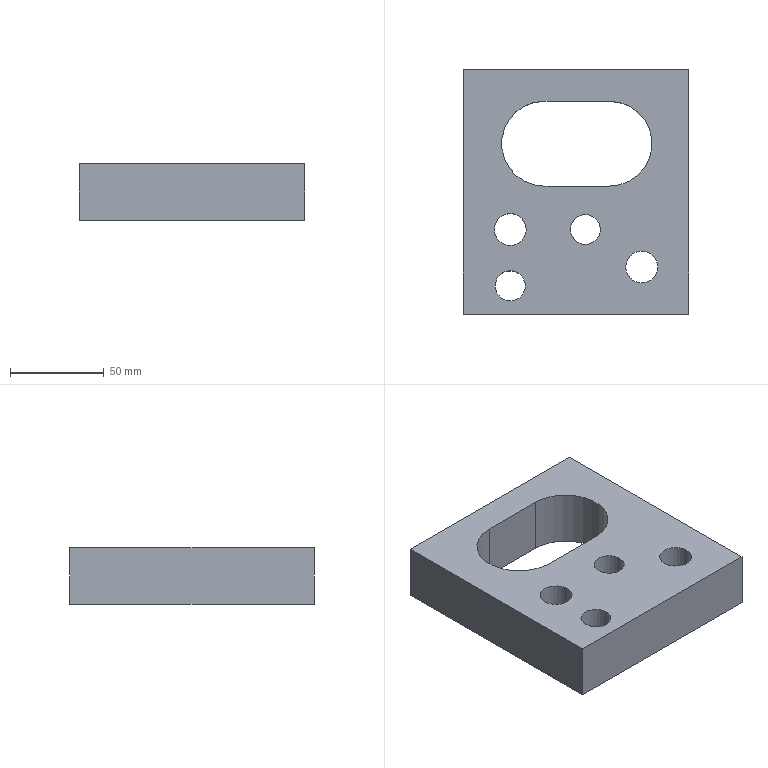Part | NX | features solid 2 | 1 solid | 18 faces | box 120 x 130 x 30 mm | volume 337905 mm3 | plane 10 | cylinder 8 | commonest cylinder face diameters 16 x2 17 x2 26 x2 45.1 x2
STEP:
#1=CARTESIAN_POINT('',(-328.,695.,180.));
#2=VERTEX_POINT('',#1);
#3=CARTESIAN_POINT('',(-320.,695.,180.));
#4=DIRECTION('',(0.,0.,-1.));
#5=DIRECTION('',(-1.,0.,0.));
#6=AXIS2_PLACEMENT_3D('',#3,#4,#5);
#7=CIRCLE('',#6,8.);
#8=EDGE_CURVE('',#2,#2,#7,.T.);
#9=ORIENTED_EDGE('',*,*,#8,.T.);
#10=EDGE_LOOP('',(#9));
#11=FACE_BOUND('',#10,.T.);
#12=CARTESIAN_POINT('',(-225.,680.,180.));
#13=VERTEX_POINT('',#12);
#14=CARTESIAN_POINT('',(-225.,810.,180.));
#15=VERTEX_POINT('',#14);
#16=CARTESIAN_POINT('',(-225.,680.,180.));
#17=DIRECTION('',(0.,1.,0.));
#18=VECTOR('',#17,1000.);
#19=LINE('',#16,#18);
#20=EDGE_CURVE('',#13,#15,#19,.T.);
#21=ORIENTED_EDGE('',*,*,#20,.T.);
#22=CARTESIAN_POINT('',(-345.,810.,180.));
#23=VERTEX_POINT('',#22);
#24=CARTESIAN_POINT('',(-385.,810.,180.));
#25=DIRECTION('',(1.,0.,0.));
#26=VECTOR('',#25,1000.);
#27=LINE('',#24,#26);
#28=EDGE_CURVE('',#23,#15,#27,.T.);
#29=ORIENTED_EDGE('',*,*,#28,.F.);
#30=CARTESIAN_POINT('',(-345.,680.,180.));
#31=VERTEX_POINT('',#30);
#32=CARTESIAN_POINT('',(-345.,810.,180.));
#33=DIRECTION('',(0.,1.,0.));
#34=VECTOR('',#33,1000.);
#35=LINE('',#32,#34);
#36=EDGE_CURVE('',#31,#23,#35,.T.);
#37=ORIENTED_EDGE('',*,*,#36,.F.);
#38=CARTESIAN_POINT('',(-385.,680.,180.));
#39=DIRECTION('',(1.,0.,0.));
#40=VECTOR('',#39,1000.);
#41=LINE('',#38,#40);
#42=EDGE_CURVE('',#31,#13,#41,.T.);
#43=ORIENTED_EDGE('',*,*,#42,.T.);
#44=EDGE_LOOP('',(#21,#29,#37,#43));
#45=FACE_BOUND('',#44,.T.);
#46=CARTESIAN_POINT('',(-311.5,725.,180.));
#47=VERTEX_POINT('',#46);
#48=CARTESIAN_POINT('',(-320.,725.,180.));
#49=DIRECTION('',(0.,0.,1.));
#50=DIRECTION('',(1.,0.,0.));
#51=AXIS2_PLACEMENT_3D('',#48,#49,#50);
#52=CIRCLE('',#51,8.5);
#53=EDGE_CURVE('',#47,#47,#52,.T.);
#54=ORIENTED_EDGE('',*,*,#53,.F.);
#55=EDGE_LOOP('',(#54));
#56=FACE_BOUND('',#55,.T.);
#57=CARTESIAN_POINT('',(-241.5,705.,180.));
#58=VERTEX_POINT('',#57);
#59=CARTESIAN_POINT('',(-250.,705.,180.));
#60=DIRECTION('',(0.,0.,1.));
#61=DIRECTION('',(1.,0.,0.));
#62=AXIS2_PLACEMENT_3D('',#59,#60,#61);
#63=CIRCLE('',#62,8.5);
#64=EDGE_CURVE('',#58,#58,#63,.T.);
#65=ORIENTED_EDGE('',*,*,#64,.F.);
#66=EDGE_LOOP('',(#65));
#67=FACE_BOUND('',#66,.T.);
#68=CARTESIAN_POINT('',(-288.,725.,180.));
#69=VERTEX_POINT('',#68);
#70=CARTESIAN_POINT('',(-280.,725.,180.));
#71=DIRECTION('',(0.,0.,-1.));
#72=DIRECTION('',(-1.,0.,0.));
#73=AXIS2_PLACEMENT_3D('',#70,#71,#72);
#74=CIRCLE('',#73,8.);
#75=EDGE_CURVE('',#69,#69,#74,.T.);
#76=ORIENTED_EDGE('',*,*,#75,.T.);
#77=EDGE_LOOP('',(#76));
#78=FACE_BOUND('',#77,.T.);
#79=CARTESIAN_POINT('',(-267.044,748.16,180.));
#80=VERTEX_POINT('',#79);
#81=CARTESIAN_POINT('',(-267.044,793.26,180.));
#82=VERTEX_POINT('',#81);
#83=CARTESIAN_POINT('',(-267.044,770.71,180.));
#84=DIRECTION('',(0.,0.,1.));
#85=DIRECTION('',(0.,-1.,0.));
#86=AXIS2_PLACEMENT_3D('',#83,#84,#85);
#87=CIRCLE('',#86,22.55);
#88=EDGE_CURVE('',#80,#82,#87,.T.);
#89=ORIENTED_EDGE('',*,*,#88,.F.);
#90=CARTESIAN_POINT('',(-302.055,748.16,180.));
#91=VERTEX_POINT('',#90);
#92=CARTESIAN_POINT('',(-267.044,748.16,180.));
#93=DIRECTION('',(-1.,0.,0.));
#94=VECTOR('',#93,1000.);
#95=LINE('',#92,#94);
#96=EDGE_CURVE('',#80,#91,#95,.T.);
#97=ORIENTED_EDGE('',*,*,#96,.T.);
#98=CARTESIAN_POINT('',(-302.055,793.26,180.));
#99=VERTEX_POINT('',#98);
#100=CARTESIAN_POINT('',(-302.055,770.71,180.));
#101=DIRECTION('',(0.,0.,1.));
#102=DIRECTION('',(0.,-1.,0.));
#103=AXIS2_PLACEMENT_3D('',#100,#101,#102);
#104=CIRCLE('',#103,22.55);
#105=EDGE_CURVE('',#99,#91,#104,.T.);
#106=ORIENTED_EDGE('',*,*,#105,.F.);
#107=CARTESIAN_POINT('',(-302.055,793.26,180.));
#108=DIRECTION('',(1.,0.,0.));
#109=VECTOR('',#108,1000.);
#110=LINE('',#107,#109);
#111=EDGE_CURVE('',#99,#82,#110,.T.);
#112=ORIENTED_EDGE('',*,*,#111,.T.);
#113=EDGE_LOOP('',(#89,#97,#106,#112));
#114=FACE_BOUND('',#113,.T.);
#115=CARTESIAN_POINT('',(-225.,810.,180.));
#116=DIRECTION('',(0.,0.,-1.));
#117=DIRECTION('',(0.,1.,0.));
#118=AXIS2_PLACEMENT_3D('',#115,#116,#117);
#119=PLANE('',#118);
#120=ADVANCED_FACE('',(#11,#45,#56,#67,#78,#114),#119,.F.);
#121=CARTESIAN_POINT('',(-312.,695.,150.));
#122=VERTEX_POINT('',#121);
#123=CARTESIAN_POINT('',(-320.,695.,150.));
#124=DIRECTION('',(0.,0.,1.));
#125=DIRECTION('',(1.,0.,0.));
#126=AXIS2_PLACEMENT_3D('',#123,#124,#125);
#127=CIRCLE('',#126,8.);
#128=EDGE_CURVE('',#122,#122,#127,.T.);
#129=ORIENTED_EDGE('',*,*,#128,.T.);
#130=EDGE_LOOP('',(#129));
#131=FACE_BOUND('',#130,.T.);
#132=CARTESIAN_POINT('',(-225.,680.,150.));
#133=VERTEX_POINT('',#132);
#134=CARTESIAN_POINT('',(-225.,810.,150.));
#135=VERTEX_POINT('',#134);
#136=CARTESIAN_POINT('',(-225.,680.,150.));
#137=DIRECTION('',(0.,1.,0.));
#138=VECTOR('',#137,1000.);
#139=LINE('',#136,#138);
#140=EDGE_CURVE('',#133,#135,#139,.T.);
#141=ORIENTED_EDGE('',*,*,#140,.F.);
#142=CARTESIAN_POINT('',(-345.,680.,150.));
#143=VERTEX_POINT('',#142);
#144=CARTESIAN_POINT('',(-385.,680.,150.));
#145=DIRECTION('',(1.,0.,0.));
#146=VECTOR('',#145,1000.);
#147=LINE('',#144,#146);
#148=EDGE_CURVE('',#143,#133,#147,.T.);
#149=ORIENTED_EDGE('',*,*,#148,.F.);
#150=CARTESIAN_POINT('',(-345.,810.,150.));
#151=VERTEX_POINT('',#150);
#152=CARTESIAN_POINT('',(-345.,810.,150.));
#153=DIRECTION('',(0.,1.,0.));
#154=VECTOR('',#153,1000.);
#155=LINE('',#152,#154);
#156=EDGE_CURVE('',#143,#151,#155,.T.);
#157=ORIENTED_EDGE('',*,*,#156,.T.);
#158=CARTESIAN_POINT('',(-385.,810.,150.));
#159=DIRECTION('',(1.,0.,0.));
#160=VECTOR('',#159,1000.);
#161=LINE('',#158,#160);
#162=EDGE_CURVE('',#151,#135,#161,.T.);
#163=ORIENTED_EDGE('',*,*,#162,.T.);
#164=EDGE_LOOP('',(#141,#149,#157,#163));
#165=FACE_BOUND('',#164,.T.);
#166=CARTESIAN_POINT('',(-307.,725.,150.));
#167=VERTEX_POINT('',#166);
#168=CARTESIAN_POINT('',(-320.,725.,150.));
#169=DIRECTION('',(0.,0.,1.));
#170=DIRECTION('',(1.,0.,0.));
#171=AXIS2_PLACEMENT_3D('',#168,#169,#170);
#172=CIRCLE('',#171,13.);
#173=EDGE_CURVE('',#167,#167,#172,.T.);
#174=ORIENTED_EDGE('',*,*,#173,.T.);
#175=EDGE_LOOP('',(#174));
#176=FACE_BOUND('',#175,.T.);
#177=CARTESIAN_POINT('',(-237.,705.,150.));
#178=VERTEX_POINT('',#177);
#179=CARTESIAN_POINT('',(-250.,705.,150.));
#180=DIRECTION('',(0.,0.,1.));
#181=DIRECTION('',(1.,0.,0.));
#182=AXIS2_PLACEMENT_3D('',#179,#180,#181);
#183=CIRCLE('',#182,13.);
#184=EDGE_CURVE('',#178,#178,#183,.T.);
#185=ORIENTED_EDGE('',*,*,#184,.T.);
#186=EDGE_LOOP('',(#185));
#187=FACE_BOUND('',#186,.T.);
#188=CARTESIAN_POINT('',(-272.,725.,150.));
#189=VERTEX_POINT('',#188);
#190=CARTESIAN_POINT('',(-280.,725.,150.));
#191=DIRECTION('',(0.,0.,1.));
#192=DIRECTION('',(1.,0.,0.));
#193=AXIS2_PLACEMENT_3D('',#190,#191,#192);
#194=CIRCLE('',#193,8.);
#195=EDGE_CURVE('',#189,#189,#194,.T.);
#196=ORIENTED_EDGE('',*,*,#195,.T.);
#197=EDGE_LOOP('',(#196));
#198=FACE_BOUND('',#197,.T.);
#199=CARTESIAN_POINT('',(-267.044,748.16,150.));
#200=VERTEX_POINT('',#199);
#201=CARTESIAN_POINT('',(-302.055,748.16,150.));
#202=VERTEX_POINT('',#201);
#203=CARTESIAN_POINT('',(-225.,748.16,150.));
#204=DIRECTION('',(-1.,0.,0.));
#205=VECTOR('',#204,1000.);
#206=LINE('',#203,#205);
#207=EDGE_CURVE('',#200,#202,#206,.T.);
#208=ORIENTED_EDGE('',*,*,#207,.F.);
#209=CARTESIAN_POINT('',(-267.044,793.26,150.));
#210=VERTEX_POINT('',#209);
#211=CARTESIAN_POINT('',(-267.044,770.71,150.));
#212=DIRECTION('',(0.,0.,-1.));
#213=DIRECTION('',(-1.,0.,0.));
#214=AXIS2_PLACEMENT_3D('',#211,#212,#213);
#215=CIRCLE('',#214,22.55);
#216=EDGE_CURVE('',#200,#210,#215,.F.);
#217=ORIENTED_EDGE('',*,*,#216,.T.);
#218=CARTESIAN_POINT('',(-302.055,793.26,150.));
#219=VERTEX_POINT('',#218);
#220=CARTESIAN_POINT('',(-225.,793.26,150.));
#221=DIRECTION('',(1.,0.,0.));
#222=VECTOR('',#221,1000.);
#223=LINE('',#220,#222);
#224=EDGE_CURVE('',#219,#210,#223,.T.);
#225=ORIENTED_EDGE('',*,*,#224,.F.);
#226=CARTESIAN_POINT('',(-302.055,770.71,150.));
#227=DIRECTION('',(0.,0.,-1.));
#228=DIRECTION('',(-1.,0.,0.));
#229=AXIS2_PLACEMENT_3D('',#226,#227,#228);
#230=CIRCLE('',#229,22.55);
#231=EDGE_CURVE('',#219,#202,#230,.F.);
#232=ORIENTED_EDGE('',*,*,#231,.T.);
#233=EDGE_LOOP('',(#208,#217,#225,#232));
#234=FACE_BOUND('',#233,.T.);
#235=CARTESIAN_POINT('',(-225.,810.,150.));
#236=DIRECTION('',(0.,0.,-1.));
#237=DIRECTION('',(0.,1.,0.));
#238=AXIS2_PLACEMENT_3D('',#235,#236,#237);
#239=PLANE('',#238);
#240=ADVANCED_FACE('',(#131,#165,#176,#187,#198,#234),#239,.T.);
#241=ORIENTED_EDGE('',*,*,#140,.T.);
#242=CARTESIAN_POINT('',(-225.,810.,180.));
#243=DIRECTION('',(0.,0.,-1.));
#244=VECTOR('',#243,1000.);
#245=LINE('',#242,#244);
#246=EDGE_CURVE('',#15,#135,#245,.T.);
#247=ORIENTED_EDGE('',*,*,#246,.F.);
#248=ORIENTED_EDGE('',*,*,#20,.F.);
#249=CARTESIAN_POINT('',(-225.,680.,180.));
#250=DIRECTION('',(0.,0.,-1.));
#251=VECTOR('',#250,1000.);
#252=LINE('',#249,#251);
#253=EDGE_CURVE('',#13,#133,#252,.T.);
#254=ORIENTED_EDGE('',*,*,#253,.T.);
#255=EDGE_LOOP('',(#241,#247,#248,#254));
#256=FACE_BOUND('',#255,.T.);
#257=CARTESIAN_POINT('',(-225.,680.,180.));
#258=DIRECTION('',(-1.,0.,0.));
#259=DIRECTION('',(0.,0.,-1.));
#260=AXIS2_PLACEMENT_3D('',#257,#258,#259);
#261=PLANE('',#260);
#262=ADVANCED_FACE('',(#256),#261,.F.);
#263=ORIENTED_EDGE('',*,*,#162,.F.);
#264=CARTESIAN_POINT('',(-345.,810.,180.));
#265=DIRECTION('',(0.,0.,-1.));
#266=VECTOR('',#265,1000.);
#267=LINE('',#264,#266);
#268=EDGE_CURVE('',#23,#151,#267,.T.);
#269=ORIENTED_EDGE('',*,*,#268,.F.);
#270=ORIENTED_EDGE('',*,*,#28,.T.);
#271=ORIENTED_EDGE('',*,*,#246,.T.);
#272=EDGE_LOOP('',(#263,#269,#270,#271));
#273=FACE_BOUND('',#272,.T.);
#274=CARTESIAN_POINT('',(-385.,810.,180.));
#275=DIRECTION('',(0.,1.,0.));
#276=DIRECTION('',(-1.,0.,0.));
#277=AXIS2_PLACEMENT_3D('',#274,#275,#276);
#278=PLANE('',#277);
#279=ADVANCED_FACE('',(#273),#278,.T.);
#280=ORIENTED_EDGE('',*,*,#156,.F.);
#281=CARTESIAN_POINT('',(-345.,680.,180.));
#282=DIRECTION('',(0.,0.,-1.));
#283=VECTOR('',#282,1000.);
#284=LINE('',#281,#283);
#285=EDGE_CURVE('',#31,#143,#284,.T.);
#286=ORIENTED_EDGE('',*,*,#285,.F.);
#287=ORIENTED_EDGE('',*,*,#36,.T.);
#288=ORIENTED_EDGE('',*,*,#268,.T.);
#289=EDGE_LOOP('',(#280,#286,#287,#288));
#290=FACE_BOUND('',#289,.T.);
#291=CARTESIAN_POINT('',(-345.,680.,180.));
#292=DIRECTION('',(-1.,0.,0.));
#293=DIRECTION('',(0.,0.,-1.));
#294=AXIS2_PLACEMENT_3D('',#291,#292,#293);
#295=PLANE('',#294);
#296=ADVANCED_FACE('',(#290),#295,.T.);
#297=ORIENTED_EDGE('',*,*,#148,.T.);
#298=ORIENTED_EDGE('',*,*,#253,.F.);
#299=ORIENTED_EDGE('',*,*,#42,.F.);
#300=ORIENTED_EDGE('',*,*,#285,.T.);
#301=EDGE_LOOP('',(#297,#298,#299,#300));
#302=FACE_BOUND('',#301,.T.);
#303=CARTESIAN_POINT('',(-385.,680.,180.));
#304=DIRECTION('',(0.,1.,0.));
#305=DIRECTION('',(-1.,0.,0.));
#306=AXIS2_PLACEMENT_3D('',#303,#304,#305);
#307=PLANE('',#306);
#308=ADVANCED_FACE('',(#302),#307,.F.);
#309=ORIENTED_EDGE('',*,*,#53,.T.);
#310=EDGE_LOOP('',(#309));
#311=FACE_BOUND('',#310,.T.);
#312=CARTESIAN_POINT('',(-311.5,725.,165.));
#313=VERTEX_POINT('',#312);
#314=CARTESIAN_POINT('',(-320.,725.,165.));
#315=DIRECTION('',(0.,0.,1.));
#316=DIRECTION('',(1.,0.,0.));
#317=AXIS2_PLACEMENT_3D('',#314,#315,#316);
#318=CIRCLE('',#317,8.5);
#319=EDGE_CURVE('',#313,#313,#318,.T.);
#320=ORIENTED_EDGE('',*,*,#319,.F.);
#321=EDGE_LOOP('',(#320));
#322=FACE_BOUND('',#321,.T.);
#323=CARTESIAN_POINT('',(-320.,725.,180.));
#324=DIRECTION('',(0.,0.,1.));
#325=DIRECTION('',(1.,0.,0.));
#326=AXIS2_PLACEMENT_3D('',#323,#324,#325);
#327=CYLINDRICAL_SURFACE('',#326,8.5);
#328=ADVANCED_FACE('',(#311,#322),#327,.F.);
#329=ORIENTED_EDGE('',*,*,#319,.T.);
#330=EDGE_LOOP('',(#329));
#331=FACE_BOUND('',#330,.T.);
#332=CARTESIAN_POINT('',(-307.,725.,165.));
#333=VERTEX_POINT('',#332);
#334=CARTESIAN_POINT('',(-320.,725.,165.));
#335=DIRECTION('',(0.,0.,1.));
#336=DIRECTION('',(1.,0.,0.));
#337=AXIS2_PLACEMENT_3D('',#334,#335,#336);
#338=CIRCLE('',#337,13.);
#339=EDGE_CURVE('',#333,#333,#338,.T.);
#340=ORIENTED_EDGE('',*,*,#339,.F.);
#341=EDGE_LOOP('',(#340));
#342=FACE_BOUND('',#341,.T.);
#343=CARTESIAN_POINT('',(-320.,725.,165.));
#344=DIRECTION('',(0.,0.,1.));
#345=DIRECTION('',(1.,0.,0.));
#346=AXIS2_PLACEMENT_3D('',#343,#344,#345);
#347=PLANE('',#346);
#348=ADVANCED_FACE('',(#331,#342),#347,.F.);
#349=ORIENTED_EDGE('',*,*,#339,.T.);
#350=EDGE_LOOP('',(#349));
#351=FACE_BOUND('',#350,.T.);
#352=ORIENTED_EDGE('',*,*,#173,.F.);
#353=EDGE_LOOP('',(#352));
#354=FACE_BOUND('',#353,.T.);
#355=CARTESIAN_POINT('',(-320.,725.,150.));
#356=DIRECTION('',(0.,0.,1.));
#357=DIRECTION('',(1.,0.,0.));
#358=AXIS2_PLACEMENT_3D('',#355,#356,#357);
#359=CYLINDRICAL_SURFACE('',#358,13.);
#360=ADVANCED_FACE('',(#351,#354),#359,.F.);
#361=ORIENTED_EDGE('',*,*,#64,.T.);
#362=EDGE_LOOP('',(#361));
#363=FACE_BOUND('',#362,.T.);
#364=CARTESIAN_POINT('',(-241.5,705.,165.));
#365=VERTEX_POINT('',#364);
#366=CARTESIAN_POINT('',(-250.,705.,165.));
#367=DIRECTION('',(0.,0.,1.));
#368=DIRECTION('',(1.,0.,0.));
#369=AXIS2_PLACEMENT_3D('',#366,#367,#368);
#370=CIRCLE('',#369,8.5);
#371=EDGE_CURVE('',#365,#365,#370,.T.);
#372=ORIENTED_EDGE('',*,*,#371,.F.);
#373=EDGE_LOOP('',(#372));
#374=FACE_BOUND('',#373,.T.);
#375=CARTESIAN_POINT('',(-250.,705.,180.));
#376=DIRECTION('',(0.,0.,1.));
#377=DIRECTION('',(1.,0.,0.));
#378=AXIS2_PLACEMENT_3D('',#375,#376,#377);
#379=CYLINDRICAL_SURFACE('',#378,8.5);
#380=ADVANCED_FACE('',(#363,#374),#379,.F.);
#381=ORIENTED_EDGE('',*,*,#371,.T.);
#382=EDGE_LOOP('',(#381));
#383=FACE_BOUND('',#382,.T.);
#384=CARTESIAN_POINT('',(-237.,705.,165.));
#385=VERTEX_POINT('',#384);
#386=CARTESIAN_POINT('',(-250.,705.,165.));
#387=DIRECTION('',(0.,0.,1.));
#388=DIRECTION('',(1.,0.,0.));
#389=AXIS2_PLACEMENT_3D('',#386,#387,#388);
#390=CIRCLE('',#389,13.);
#391=EDGE_CURVE('',#385,#385,#390,.T.);
#392=ORIENTED_EDGE('',*,*,#391,.F.);
#393=EDGE_LOOP('',(#392));
#394=FACE_BOUND('',#393,.T.);
#395=CARTESIAN_POINT('',(-250.,705.,165.));
#396=DIRECTION('',(0.,0.,1.));
#397=DIRECTION('',(1.,0.,0.));
#398=AXIS2_PLACEMENT_3D('',#395,#396,#397);
#399=PLANE('',#398);
#400=ADVANCED_FACE('',(#383,#394),#399,.F.);
#401=ORIENTED_EDGE('',*,*,#391,.T.);
#402=EDGE_LOOP('',(#401));
#403=FACE_BOUND('',#402,.T.);
#404=ORIENTED_EDGE('',*,*,#184,.F.);
#405=EDGE_LOOP('',(#404));
#406=FACE_BOUND('',#405,.T.);
#407=CARTESIAN_POINT('',(-250.,705.,150.));
#408=DIRECTION('',(0.,0.,1.));
#409=DIRECTION('',(1.,0.,0.));
#410=AXIS2_PLACEMENT_3D('',#407,#408,#409);
#411=CYLINDRICAL_SURFACE('',#410,13.);
#412=ADVANCED_FACE('',(#403,#406),#411,.F.);
#413=ORIENTED_EDGE('',*,*,#195,.F.);
#414=EDGE_LOOP('',(#413));
#415=FACE_BOUND('',#414,.T.);
#416=ORIENTED_EDGE('',*,*,#75,.F.);
#417=EDGE_LOOP('',(#416));
#418=FACE_BOUND('',#417,.T.);
#419=CARTESIAN_POINT('',(-280.,725.,150.));
#420=DIRECTION('',(0.,0.,1.));
#421=DIRECTION('',(1.,0.,0.));
#422=AXIS2_PLACEMENT_3D('',#419,#420,#421);
#423=CYLINDRICAL_SURFACE('',#422,8.);
#424=ADVANCED_FACE('',(#415,#418),#423,.F.);
#425=CARTESIAN_POINT('',(-267.044,748.16,200.));
#426=DIRECTION('',(0.,0.,-1.));
#427=VECTOR('',#426,1000.);
#428=LINE('',#425,#427);
#429=EDGE_CURVE('',#80,#200,#428,.T.);
#430=ORIENTED_EDGE('',*,*,#429,.F.);
#431=ORIENTED_EDGE('',*,*,#88,.T.);
#432=CARTESIAN_POINT('',(-267.044,793.26,200.));
#433=DIRECTION('',(0.,0.,-1.));
#434=VECTOR('',#433,1000.);
#435=LINE('',#432,#434);
#436=EDGE_CURVE('',#82,#210,#435,.T.);
#437=ORIENTED_EDGE('',*,*,#436,.T.);
#438=ORIENTED_EDGE('',*,*,#216,.F.);
#439=EDGE_LOOP('',(#430,#431,#437,#438));
#440=FACE_BOUND('',#439,.T.);
#441=CARTESIAN_POINT('',(-267.044,770.71,200.));
#442=DIRECTION('',(0.,0.,-1.));
#443=DIRECTION('',(0.,1.,0.));
#444=AXIS2_PLACEMENT_3D('',#441,#442,#443);
#445=CYLINDRICAL_SURFACE('',#444,22.55);
#446=ADVANCED_FACE('',(#440),#445,.F.);
#447=ORIENTED_EDGE('',*,*,#224,.T.);
#448=ORIENTED_EDGE('',*,*,#436,.F.);
#449=ORIENTED_EDGE('',*,*,#111,.F.);
#450=CARTESIAN_POINT('',(-302.055,793.26,200.));
#451=DIRECTION('',(0.,0.,-1.));
#452=VECTOR('',#451,1000.);
#453=LINE('',#450,#452);
#454=EDGE_CURVE('',#99,#219,#453,.T.);
#455=ORIENTED_EDGE('',*,*,#454,.T.);
#456=EDGE_LOOP('',(#447,#448,#449,#455));
#457=FACE_BOUND('',#456,.T.);
#458=CARTESIAN_POINT('',(-302.055,793.26,200.));
#459=DIRECTION('',(0.,1.,0.));
#460=DIRECTION('',(0.,0.,1.));
#461=AXIS2_PLACEMENT_3D('',#458,#459,#460);
#462=PLANE('',#461);
#463=ADVANCED_FACE('',(#457),#462,.F.);
#464=ORIENTED_EDGE('',*,*,#454,.F.);
#465=ORIENTED_EDGE('',*,*,#105,.T.);
#466=CARTESIAN_POINT('',(-302.055,748.16,200.));
#467=DIRECTION('',(0.,0.,-1.));
#468=VECTOR('',#467,1000.);
#469=LINE('',#466,#468);
#470=EDGE_CURVE('',#91,#202,#469,.T.);
#471=ORIENTED_EDGE('',*,*,#470,.T.);
#472=ORIENTED_EDGE('',*,*,#231,.F.);
#473=EDGE_LOOP('',(#464,#465,#471,#472));
#474=FACE_BOUND('',#473,.T.);
#475=CARTESIAN_POINT('',(-302.055,770.71,200.));
#476=DIRECTION('',(0.,0.,-1.));
#477=DIRECTION('',(0.,1.,0.));
#478=AXIS2_PLACEMENT_3D('',#475,#476,#477);
#479=CYLINDRICAL_SURFACE('',#478,22.55);
#480=ADVANCED_FACE('',(#474),#479,.F.);
#481=ORIENTED_EDGE('',*,*,#207,.T.);
#482=ORIENTED_EDGE('',*,*,#470,.F.);
#483=ORIENTED_EDGE('',*,*,#96,.F.);
#484=ORIENTED_EDGE('',*,*,#429,.T.);
#485=EDGE_LOOP('',(#481,#482,#483,#484));
#486=FACE_BOUND('',#485,.T.);
#487=CARTESIAN_POINT('',(-267.044,748.16,200.));
#488=DIRECTION('',(0.,-1.,0.));
#489=DIRECTION('',(0.,0.,-1.));
#490=AXIS2_PLACEMENT_3D('',#487,#488,#489);
#491=PLANE('',#490);
#492=ADVANCED_FACE('',(#486),#491,.F.);
#493=ORIENTED_EDGE('',*,*,#128,.F.);
#494=EDGE_LOOP('',(#493));
#495=FACE_BOUND('',#494,.T.);
#496=ORIENTED_EDGE('',*,*,#8,.F.);
#497=EDGE_LOOP('',(#496));
#498=FACE_BOUND('',#497,.T.);
#499=CARTESIAN_POINT('',(-320.,695.,150.));
#500=DIRECTION('',(0.,0.,1.));
#501=DIRECTION('',(1.,0.,0.));
#502=AXIS2_PLACEMENT_3D('',#499,#500,#501);
#503=CYLINDRICAL_SURFACE('',#502,8.);
#504=ADVANCED_FACE('',(#495,#498),#503,.F.);
#505=CLOSED_SHELL('',(#120,#240,#262,#279,#296,#308,#328,#348,#360,#380,#400,#412,#424,#446,#463,#480,#492,#504));
#506=MANIFOLD_SOLID_BREP('',#505);
#507=(LENGTH_UNIT()NAMED_UNIT(*)SI_UNIT(.MILLI.,.METRE.));
#508=UNCERTAINTY_MEASURE_WITH_UNIT(LENGTH_MEASURE(0.00001),#507,'','');
#509=(NAMED_UNIT(*)PLANE_ANGLE_UNIT()SI_UNIT($,.RADIAN.));
#510=(NAMED_UNIT(*)SI_UNIT($,.STERADIAN.)SOLID_ANGLE_UNIT());
#511=(GEOMETRIC_REPRESENTATION_CONTEXT(3)GLOBAL_UNCERTAINTY_ASSIGNED_CONTEXT((#508))GLOBAL_UNIT_ASSIGNED_CONTEXT((#507,#509,#510))REPRESENTATION_CONTEXT('',''));
#512=ADVANCED_BREP_SHAPE_REPRESENTATION('',(#506),#511);